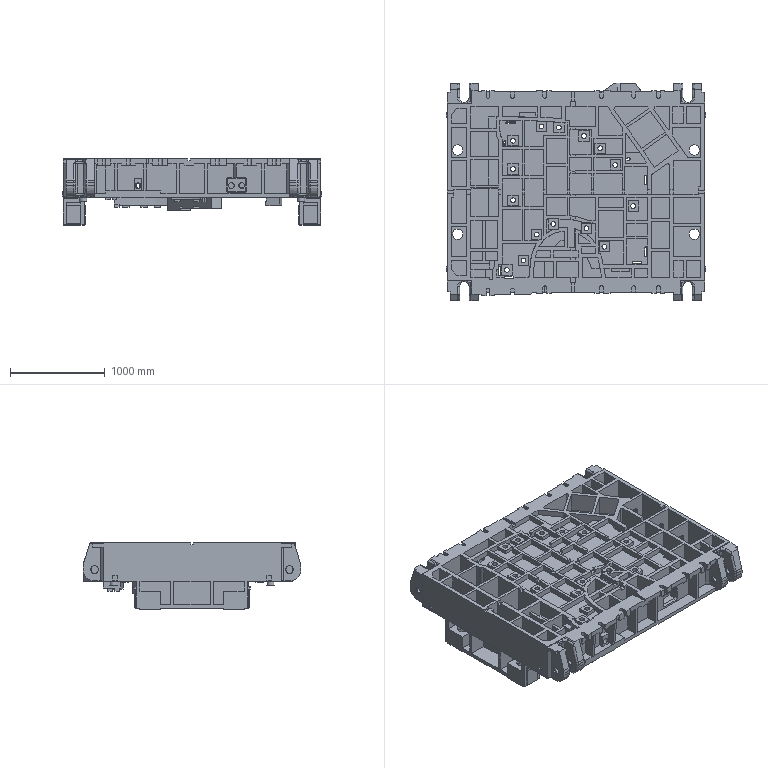Part | NX | features solid 2 | 1 solid | 2257 faces | box 2740 x 2301 x 705 mm | volume 883945977 mm3 | plane 1855 | cylinder 317 | spline 57 | torus 28 | commonest cylinder face diameters 40 x65 80 x57 83 x48 20 x32 79 x16 30 x14